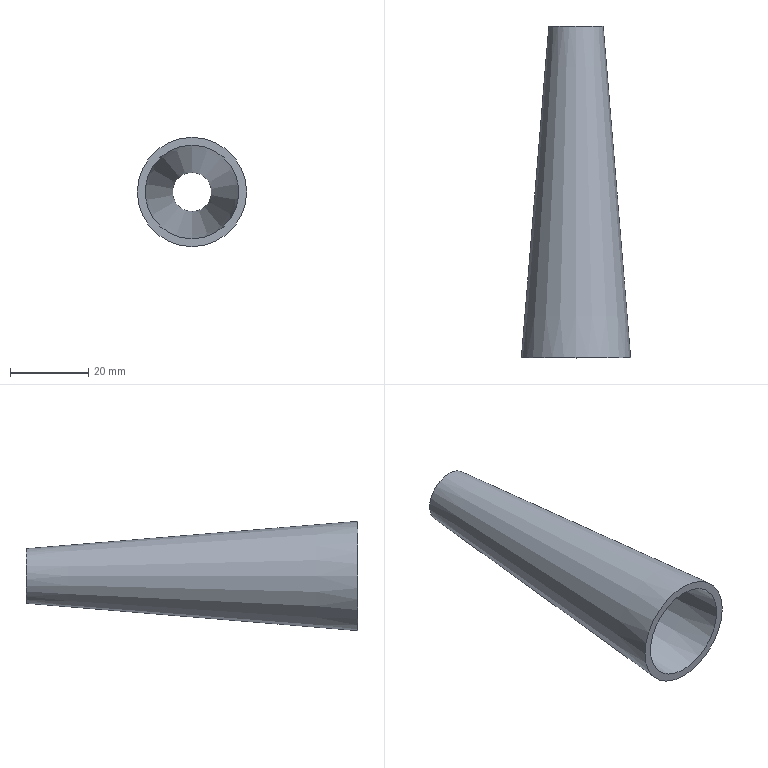Part | NX | features DATUM_CSYS 2, SWP104 2, SKETCH 1 | 1 solid | 4 faces | box 28 x 85 x 28 mm | volume 10147 mm3 | plane 2 | cone 2
STEP:
#1=CARTESIAN_POINT('',(0.,85.,5.));
#2=VERTEX_POINT('',#1);
#3=CARTESIAN_POINT('',(0.,85.,0.));
#4=DIRECTION('',(0.,1.,0.));
#5=DIRECTION('',(0.,0.,1.));
#6=AXIS2_PLACEMENT_3D('',#3,#4,#5);
#7=CIRCLE('',#6,5.);
#8=EDGE_CURVE('',#2,#2,#7,.T.);
#9=ORIENTED_EDGE('',*,*,#8,.F.);
#10=EDGE_LOOP('',(#9));
#11=FACE_BOUND('',#10,.T.);
#12=CARTESIAN_POINT('',(0.,85.,7.));
#13=VERTEX_POINT('',#12);
#14=CARTESIAN_POINT('',(0.,85.,0.));
#15=DIRECTION('',(0.,1.,0.));
#16=DIRECTION('',(0.,0.,1.));
#17=AXIS2_PLACEMENT_3D('',#14,#15,#16);
#18=CIRCLE('',#17,7.);
#19=EDGE_CURVE('',#13,#13,#18,.T.);
#20=ORIENTED_EDGE('',*,*,#19,.T.);
#21=EDGE_LOOP('',(#20));
#22=FACE_BOUND('',#21,.T.);
#23=CARTESIAN_POINT('',(7.,85.,0.));
#24=DIRECTION('',(0.,-1.,0.));
#25=DIRECTION('',(0.,0.,-1.));
#26=AXIS2_PLACEMENT_3D('',#23,#24,#25);
#27=PLANE('',#26);
#28=ADVANCED_FACE('',(#11,#22),#27,.F.);
#29=CARTESIAN_POINT('',(0.,0.,12.));
#30=VERTEX_POINT('',#29);
#31=CARTESIAN_POINT('',(0.,0.,0.));
#32=DIRECTION('',(0.,1.,0.));
#33=DIRECTION('',(0.,0.,1.));
#34=AXIS2_PLACEMENT_3D('',#31,#32,#33);
#35=CIRCLE('',#34,12.);
#36=EDGE_CURVE('',#30,#30,#35,.T.);
#37=ORIENTED_EDGE('',*,*,#36,.F.);
#38=EDGE_LOOP('',(#37));
#39=FACE_BOUND('',#38,.T.);
#40=ORIENTED_EDGE('',*,*,#8,.T.);
#41=EDGE_LOOP('',(#40));
#42=FACE_BOUND('',#41,.T.);
#43=CARTESIAN_POINT('',(0.,85.,0.));
#44=DIRECTION('',(0.,-1.,0.));
#45=DIRECTION('',(0.,0.,-1.));
#46=AXIS2_PLACEMENT_3D('',#43,#44,#45);
#47=CONICAL_SURFACE('',#46,5.,0.08217);
#48=ADVANCED_FACE('',(#39,#42),#47,.F.);
#49=CARTESIAN_POINT('',(0.,0.,14.));
#50=VERTEX_POINT('',#49);
#51=CARTESIAN_POINT('',(0.,0.,0.));
#52=DIRECTION('',(0.,1.,0.));
#53=DIRECTION('',(0.,0.,1.));
#54=AXIS2_PLACEMENT_3D('',#51,#52,#53);
#55=CIRCLE('',#54,14.);
#56=EDGE_CURVE('',#50,#50,#55,.T.);
#57=ORIENTED_EDGE('',*,*,#56,.F.);
#58=EDGE_LOOP('',(#57));
#59=FACE_BOUND('',#58,.T.);
#60=ORIENTED_EDGE('',*,*,#36,.T.);
#61=EDGE_LOOP('',(#60));
#62=FACE_BOUND('',#61,.T.);
#63=CARTESIAN_POINT('',(12.,0.,0.));
#64=DIRECTION('',(0.,1.,0.));
#65=DIRECTION('',(0.,0.,1.));
#66=AXIS2_PLACEMENT_3D('',#63,#64,#65);
#67=PLANE('',#66);
#68=ADVANCED_FACE('',(#59,#62),#67,.F.);
#69=ORIENTED_EDGE('',*,*,#19,.F.);
#70=EDGE_LOOP('',(#69));
#71=FACE_BOUND('',#70,.T.);
#72=ORIENTED_EDGE('',*,*,#56,.T.);
#73=EDGE_LOOP('',(#72));
#74=FACE_BOUND('',#73,.T.);
#75=CARTESIAN_POINT('',(0.,0.,0.));
#76=DIRECTION('',(0.,-1.,0.));
#77=DIRECTION('',(0.,0.,-1.));
#78=AXIS2_PLACEMENT_3D('',#75,#76,#77);
#79=CONICAL_SURFACE('',#78,14.,0.08217);
#80=ADVANCED_FACE('',(#71,#74),#79,.T.);
#81=CLOSED_SHELL('',(#28,#48,#68,#80));
#82=MANIFOLD_SOLID_BREP('',#81);
#83=(LENGTH_UNIT()NAMED_UNIT(*)SI_UNIT(.MILLI.,.METRE.));
#84=UNCERTAINTY_MEASURE_WITH_UNIT(LENGTH_MEASURE(0.00001),#83,'','');
#85=(NAMED_UNIT(*)PLANE_ANGLE_UNIT()SI_UNIT($,.RADIAN.));
#86=(NAMED_UNIT(*)SI_UNIT($,.STERADIAN.)SOLID_ANGLE_UNIT());
#87=(GEOMETRIC_REPRESENTATION_CONTEXT(3)GLOBAL_UNCERTAINTY_ASSIGNED_CONTEXT((#84))GLOBAL_UNIT_ASSIGNED_CONTEXT((#83,#85,#86))REPRESENTATION_CONTEXT('',''));
#88=ADVANCED_BREP_SHAPE_REPRESENTATION('',(#82),#87);